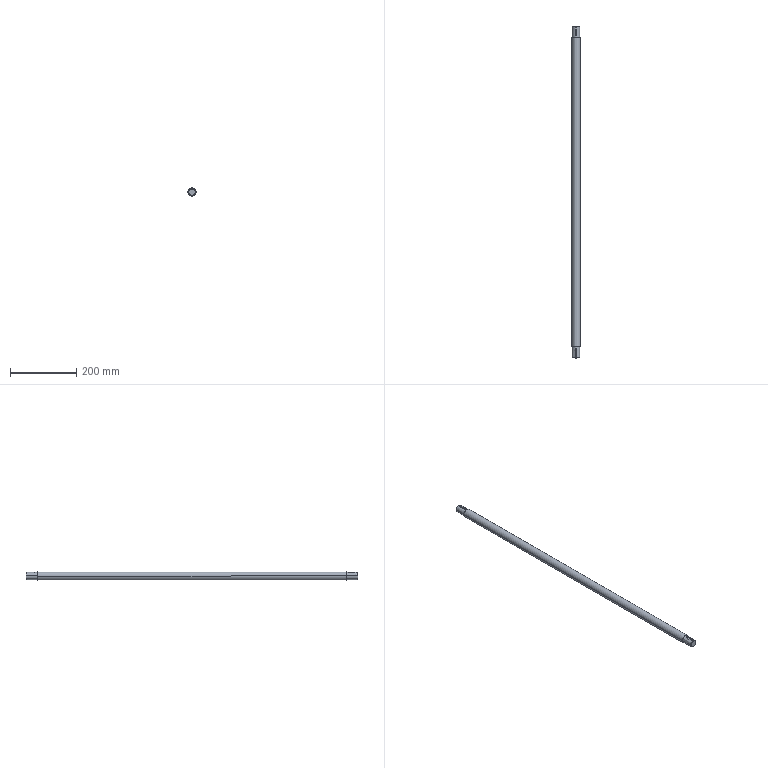Part | STEP file | CONNECTING.SHAFT.stp | 1 solid | 28 faces | box 25 x 1000 x 25 mm | volume 481905 mm3 | spline 12 | cylinder 8 | plane 6 | cone 2 | commonest cylinder face diameters 6 x4 22 x2 25 x2